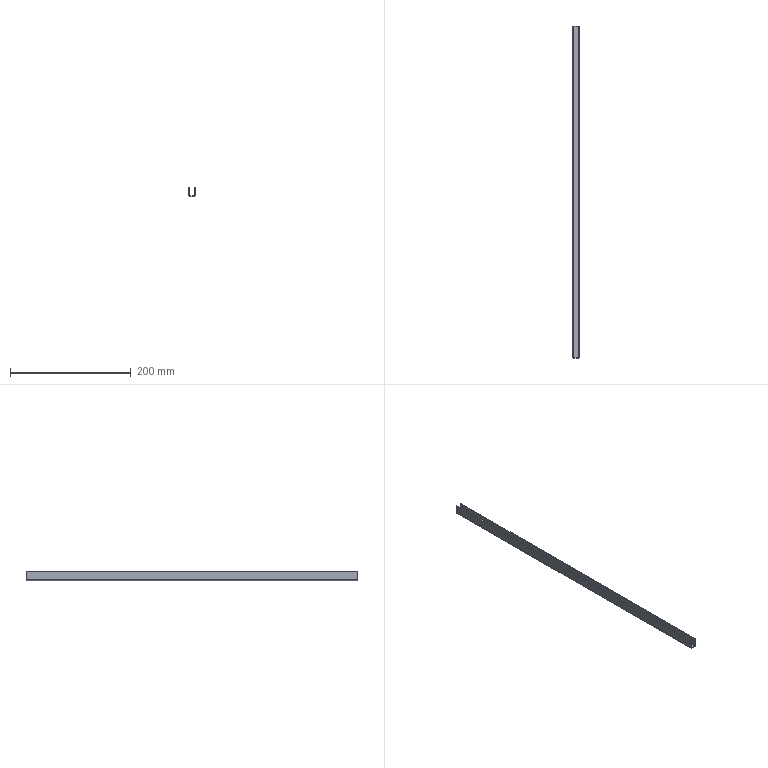Part | SolidWorks | features EdgeFlange 1, FlatPattern 1, SMBaseFlange 1, SheetMetal 1 | 1 solid | 22 faces | box 10.4 x 550 x 15 mm | volume 24485 mm3 | plane 18 | cylinder 4 | commonest cylinder face diameters 0.9 x2 3.3 x2
STEP:
#1=CARTESIAN_POINT('',(-11.654,-507.682,1.2));
#2=VERTEX_POINT('',#1);
#3=CARTESIAN_POINT('',(-11.654,-507.682,0.));
#4=VERTEX_POINT('',#3);
#5=CARTESIAN_POINT('',(-11.654,-507.682,1.2));
#6=DIRECTION('',(0.,0.,-1.));
#7=VECTOR('',#6,1000.);
#8=LINE('',#5,#7);
#9=EDGE_CURVE('',#2,#4,#8,.T.);
#10=ORIENTED_EDGE('',*,*,#9,.T.);
#11=CARTESIAN_POINT('',(-4.554,-507.682,0.));
#12=VERTEX_POINT('',#11);
#13=CARTESIAN_POINT('',(-13.304,-507.682,0.));
#14=DIRECTION('',(1.,0.,0.));
#15=VECTOR('',#14,1000.);
#16=LINE('',#13,#15);
#17=EDGE_CURVE('',#4,#12,#16,.T.);
#18=ORIENTED_EDGE('',*,*,#17,.T.);
#19=CARTESIAN_POINT('',(-4.554,-507.682,1.2));
#20=VERTEX_POINT('',#19);
#21=CARTESIAN_POINT('',(-4.554,-507.682,1.2));
#22=DIRECTION('',(0.,0.,-1.));
#23=VECTOR('',#22,1000.);
#24=LINE('',#21,#23);
#25=EDGE_CURVE('',#20,#12,#24,.T.);
#26=ORIENTED_EDGE('',*,*,#25,.F.);
#27=CARTESIAN_POINT('',(-13.304,-507.682,1.2));
#28=DIRECTION('',(1.,0.,0.));
#29=VECTOR('',#28,1000.);
#30=LINE('',#27,#29);
#31=EDGE_CURVE('',#2,#20,#30,.T.);
#32=ORIENTED_EDGE('',*,*,#31,.F.);
#33=EDGE_LOOP('',(#10,#18,#26,#32));
#34=FACE_OUTER_BOUND('',#33,.T.);
#35=CARTESIAN_POINT('',(-13.304,-507.682,1.2));
#36=DIRECTION('',(0.,1.,0.));
#37=DIRECTION('',(0.,0.,1.));
#38=AXIS2_PLACEMENT_3D('',#35,#36,#37);
#39=PLANE('',#38);
#40=ADVANCED_FACE('',(#34),#39,.F.);
#41=CARTESIAN_POINT('',(-11.654,42.318,1.2));
#42=VERTEX_POINT('',#41);
#43=CARTESIAN_POINT('',(-11.654,42.318,0.));
#44=VERTEX_POINT('',#43);
#45=CARTESIAN_POINT('',(-11.654,42.318,1.2));
#46=DIRECTION('',(0.,0.,-1.));
#47=VECTOR('',#46,1000.);
#48=LINE('',#45,#47);
#49=EDGE_CURVE('',#42,#44,#48,.T.);
#50=ORIENTED_EDGE('',*,*,#49,.F.);
#51=CARTESIAN_POINT('',(-4.554,42.318,1.2));
#52=VERTEX_POINT('',#51);
#53=CARTESIAN_POINT('',(-13.304,42.318,1.2));
#54=DIRECTION('',(-1.,0.,0.));
#55=VECTOR('',#54,1000.);
#56=LINE('',#53,#55);
#57=EDGE_CURVE('',#52,#42,#56,.T.);
#58=ORIENTED_EDGE('',*,*,#57,.F.);
#59=CARTESIAN_POINT('',(-4.554,42.318,0.));
#60=VERTEX_POINT('',#59);
#61=CARTESIAN_POINT('',(-4.554,42.318,1.2));
#62=DIRECTION('',(0.,0.,-1.));
#63=VECTOR('',#62,1000.);
#64=LINE('',#61,#63);
#65=EDGE_CURVE('',#52,#60,#64,.T.);
#66=ORIENTED_EDGE('',*,*,#65,.T.);
#67=CARTESIAN_POINT('',(-13.304,42.318,0.));
#68=DIRECTION('',(-1.,0.,0.));
#69=VECTOR('',#68,1000.);
#70=LINE('',#67,#69);
#71=EDGE_CURVE('',#60,#44,#70,.T.);
#72=ORIENTED_EDGE('',*,*,#71,.T.);
#73=EDGE_LOOP('',(#50,#58,#66,#72));
#74=FACE_OUTER_BOUND('',#73,.T.);
#75=CARTESIAN_POINT('',(-13.304,42.318,1.2));
#76=DIRECTION('',(0.,-1.,0.));
#77=DIRECTION('',(0.,0.,-1.));
#78=AXIS2_PLACEMENT_3D('',#75,#76,#77);
#79=PLANE('',#78);
#80=ADVANCED_FACE('',(#74),#79,.F.);
#81=ORIENTED_EDGE('',*,*,#57,.T.);
#82=CARTESIAN_POINT('',(-11.654,-507.682,1.2));
#83=DIRECTION('',(0.,1.,0.));
#84=VECTOR('',#83,1000.);
#85=LINE('',#82,#84);
#86=EDGE_CURVE('',#2,#42,#85,.T.);
#87=ORIENTED_EDGE('',*,*,#86,.F.);
#88=ORIENTED_EDGE('',*,*,#31,.T.);
#89=CARTESIAN_POINT('',(-4.554,42.318,1.2));
#90=DIRECTION('',(0.,-1.,0.));
#91=VECTOR('',#90,1000.);
#92=LINE('',#89,#91);
#93=EDGE_CURVE('',#52,#20,#92,.T.);
#94=ORIENTED_EDGE('',*,*,#93,.F.);
#95=EDGE_LOOP('',(#81,#87,#88,#94));
#96=FACE_OUTER_BOUND('',#95,.T.);
#97=CARTESIAN_POINT('',(-13.304,-507.682,1.2));
#98=DIRECTION('',(0.,0.,1.));
#99=DIRECTION('',(1.,0.,0.));
#100=AXIS2_PLACEMENT_3D('',#97,#98,#99);
#101=PLANE('',#100);
#102=ADVANCED_FACE('',(#96),#101,.T.);
#103=CARTESIAN_POINT('',(-11.654,-507.682,0.));
#104=DIRECTION('',(0.,1.,0.));
#105=VECTOR('',#104,1000.);
#106=LINE('',#103,#105);
#107=EDGE_CURVE('',#4,#44,#106,.T.);
#108=ORIENTED_EDGE('',*,*,#107,.T.);
#109=ORIENTED_EDGE('',*,*,#71,.F.);
#110=CARTESIAN_POINT('',(-4.554,42.318,0.));
#111=DIRECTION('',(0.,-1.,0.));
#112=VECTOR('',#111,1000.);
#113=LINE('',#110,#112);
#114=EDGE_CURVE('',#60,#12,#113,.T.);
#115=ORIENTED_EDGE('',*,*,#114,.T.);
#116=ORIENTED_EDGE('',*,*,#17,.F.);
#117=EDGE_LOOP('',(#108,#109,#115,#116));
#118=FACE_OUTER_BOUND('',#117,.T.);
#119=CARTESIAN_POINT('',(-13.304,-507.682,0.));
#120=DIRECTION('',(0.,0.,1.));
#121=DIRECTION('',(1.,0.,0.));
#122=AXIS2_PLACEMENT_3D('',#119,#120,#121);
#123=PLANE('',#122);
#124=ADVANCED_FACE('',(#118),#123,.F.);
#125=CARTESIAN_POINT('',(-4.104,-507.682,1.65));
#126=VERTEX_POINT('',#125);
#127=CARTESIAN_POINT('',(-2.904,-507.682,1.65));
#128=VERTEX_POINT('',#127);
#129=CARTESIAN_POINT('',(-2.904,-507.682,1.65));
#130=DIRECTION('',(1.,0.,0.));
#131=VECTOR('',#130,1000.);
#132=LINE('',#129,#131);
#133=EDGE_CURVE('',#126,#128,#132,.T.);
#134=ORIENTED_EDGE('',*,*,#133,.F.);
#135=CARTESIAN_POINT('',(-4.554,-507.682,1.65));
#136=DIRECTION('',(0.,-1.,0.));
#137=DIRECTION('',(0.,0.,1.));
#138=AXIS2_PLACEMENT_3D('',#135,#136,#137);
#139=CIRCLE('',#138,0.45);
#140=EDGE_CURVE('',#20,#126,#139,.T.);
#141=ORIENTED_EDGE('',*,*,#140,.F.);
#142=ORIENTED_EDGE('',*,*,#25,.T.);
#143=CARTESIAN_POINT('',(-4.554,-507.682,1.65));
#144=DIRECTION('',(0.,-1.,0.));
#145=DIRECTION('',(0.,0.,1.));
#146=AXIS2_PLACEMENT_3D('',#143,#144,#145);
#147=CIRCLE('',#146,1.65);
#148=EDGE_CURVE('',#12,#128,#147,.T.);
#149=ORIENTED_EDGE('',*,*,#148,.T.);
#150=EDGE_LOOP('',(#134,#141,#142,#149));
#151=FACE_OUTER_BOUND('',#150,.T.);
#152=CARTESIAN_POINT('',(-4.554,-507.682,1.65));
#153=DIRECTION('',(0.,-1.,0.));
#154=DIRECTION('',(0.,0.,-1.));
#155=AXIS2_PLACEMENT_3D('',#152,#153,#154);
#156=PLANE('',#155);
#157=ADVANCED_FACE('',(#151),#156,.T.);
#158=ORIENTED_EDGE('',*,*,#114,.F.);
#159=CARTESIAN_POINT('',(-2.904,42.318,1.65));
#160=VERTEX_POINT('',#159);
#161=CARTESIAN_POINT('',(-4.554,42.318,1.65));
#162=DIRECTION('',(0.,1.,0.));
#163=DIRECTION('',(0.,0.,1.));
#164=AXIS2_PLACEMENT_3D('',#161,#162,#163);
#165=CIRCLE('',#164,1.65);
#166=EDGE_CURVE('',#160,#60,#165,.T.);
#167=ORIENTED_EDGE('',*,*,#166,.F.);
#168=CARTESIAN_POINT('',(-2.904,-507.682,1.65));
#169=DIRECTION('',(0.,-1.,0.));
#170=VECTOR('',#169,1000.);
#171=LINE('',#168,#170);
#172=EDGE_CURVE('',#160,#128,#171,.T.);
#173=ORIENTED_EDGE('',*,*,#172,.T.);
#174=ORIENTED_EDGE('',*,*,#148,.F.);
#175=EDGE_LOOP('',(#158,#167,#173,#174));
#176=FACE_OUTER_BOUND('',#175,.T.);
#177=CARTESIAN_POINT('',(-4.554,42.318,1.65));
#178=DIRECTION('',(0.,1.,0.));
#179=DIRECTION('',(1.,0.,0.));
#180=AXIS2_PLACEMENT_3D('',#177,#178,#179);
#181=CYLINDRICAL_SURFACE('',#180,1.65);
#182=ADVANCED_FACE('',(#176),#181,.T.);
#183=CARTESIAN_POINT('',(-4.104,42.318,1.65));
#184=VERTEX_POINT('',#183);
#185=CARTESIAN_POINT('',(-4.554,42.318,1.65));
#186=DIRECTION('',(0.,1.,0.));
#187=DIRECTION('',(0.,0.,1.));
#188=AXIS2_PLACEMENT_3D('',#185,#186,#187);
#189=CIRCLE('',#188,0.45);
#190=EDGE_CURVE('',#184,#52,#189,.T.);
#191=ORIENTED_EDGE('',*,*,#190,.F.);
#192=CARTESIAN_POINT('',(-4.104,42.318,1.65));
#193=DIRECTION('',(1.,0.,0.));
#194=VECTOR('',#193,1000.);
#195=LINE('',#192,#194);
#196=EDGE_CURVE('',#184,#160,#195,.T.);
#197=ORIENTED_EDGE('',*,*,#196,.T.);
#198=ORIENTED_EDGE('',*,*,#166,.T.);
#199=ORIENTED_EDGE('',*,*,#65,.F.);
#200=EDGE_LOOP('',(#191,#197,#198,#199));
#201=FACE_OUTER_BOUND('',#200,.T.);
#202=CARTESIAN_POINT('',(-4.554,42.318,1.65));
#203=DIRECTION('',(0.,-1.,0.));
#204=DIRECTION('',(0.,0.,-1.));
#205=AXIS2_PLACEMENT_3D('',#202,#203,#204);
#206=PLANE('',#205);
#207=ADVANCED_FACE('',(#201),#206,.F.);
#208=ORIENTED_EDGE('',*,*,#93,.T.);
#209=ORIENTED_EDGE('',*,*,#140,.T.);
#210=CARTESIAN_POINT('',(-4.104,-507.682,1.65));
#211=DIRECTION('',(0.,1.,0.));
#212=VECTOR('',#211,1000.);
#213=LINE('',#210,#212);
#214=EDGE_CURVE('',#126,#184,#213,.T.);
#215=ORIENTED_EDGE('',*,*,#214,.T.);
#216=ORIENTED_EDGE('',*,*,#190,.T.);
#217=EDGE_LOOP('',(#208,#209,#215,#216));
#218=FACE_OUTER_BOUND('',#217,.T.);
#219=CARTESIAN_POINT('',(-4.554,42.318,1.65));
#220=DIRECTION('',(0.,1.,0.));
#221=DIRECTION('',(1.,0.,0.));
#222=AXIS2_PLACEMENT_3D('',#219,#220,#221);
#223=CYLINDRICAL_SURFACE('',#222,0.45);
#224=ADVANCED_FACE('',(#218),#223,.F.);
#225=ORIENTED_EDGE('',*,*,#196,.F.);
#226=CARTESIAN_POINT('',(-4.104,42.318,15.));
#227=VERTEX_POINT('',#226);
#228=CARTESIAN_POINT('',(-4.104,42.318,15.));
#229=DIRECTION('',(0.,0.,1.));
#230=VECTOR('',#229,1000.);
#231=LINE('',#228,#230);
#232=EDGE_CURVE('',#184,#227,#231,.T.);
#233=ORIENTED_EDGE('',*,*,#232,.T.);
#234=CARTESIAN_POINT('',(-2.904,42.318,15.));
#235=VERTEX_POINT('',#234);
#236=CARTESIAN_POINT('',(-2.904,42.318,15.));
#237=DIRECTION('',(-1.,0.,0.));
#238=VECTOR('',#237,1000.);
#239=LINE('',#236,#238);
#240=EDGE_CURVE('',#235,#227,#239,.T.);
#241=ORIENTED_EDGE('',*,*,#240,.F.);
#242=CARTESIAN_POINT('',(-2.904,42.318,1.2));
#243=DIRECTION('',(0.,0.,1.));
#244=VECTOR('',#243,1000.);
#245=LINE('',#242,#244);
#246=EDGE_CURVE('',#160,#235,#245,.T.);
#247=ORIENTED_EDGE('',*,*,#246,.F.);
#248=EDGE_LOOP('',(#225,#233,#241,#247));
#249=FACE_OUTER_BOUND('',#248,.T.);
#250=CARTESIAN_POINT('',(-2.904,42.318,15.));
#251=DIRECTION('',(0.,-1.,0.));
#252=DIRECTION('',(1.,0.,0.));
#253=AXIS2_PLACEMENT_3D('',#250,#251,#252);
#254=PLANE('',#253);
#255=ADVANCED_FACE('',(#249),#254,.F.);
#256=ORIENTED_EDGE('',*,*,#133,.T.);
#257=CARTESIAN_POINT('',(-2.904,-507.682,15.));
#258=VERTEX_POINT('',#257);
#259=CARTESIAN_POINT('',(-2.904,-507.682,1.2));
#260=DIRECTION('',(0.,0.,-1.));
#261=VECTOR('',#260,1000.);
#262=LINE('',#259,#261);
#263=EDGE_CURVE('',#258,#128,#262,.T.);
#264=ORIENTED_EDGE('',*,*,#263,.F.);
#265=CARTESIAN_POINT('',(-4.104,-507.682,15.));
#266=VERTEX_POINT('',#265);
#267=CARTESIAN_POINT('',(-2.904,-507.682,15.));
#268=DIRECTION('',(-1.,0.,0.));
#269=VECTOR('',#268,1000.);
#270=LINE('',#267,#269);
#271=EDGE_CURVE('',#258,#266,#270,.T.);
#272=ORIENTED_EDGE('',*,*,#271,.T.);
#273=CARTESIAN_POINT('',(-4.104,-507.682,1.2));
#274=DIRECTION('',(0.,0.,-1.));
#275=VECTOR('',#274,1000.);
#276=LINE('',#273,#275);
#277=EDGE_CURVE('',#266,#126,#276,.T.);
#278=ORIENTED_EDGE('',*,*,#277,.T.);
#279=EDGE_LOOP('',(#256,#264,#272,#278));
#280=FACE_OUTER_BOUND('',#279,.T.);
#281=CARTESIAN_POINT('',(-2.904,-507.682,1.2));
#282=DIRECTION('',(0.,1.,0.));
#283=DIRECTION('',(-1.,0.,0.));
#284=AXIS2_PLACEMENT_3D('',#281,#282,#283);
#285=PLANE('',#284);
#286=ADVANCED_FACE('',(#280),#285,.F.);
#287=ORIENTED_EDGE('',*,*,#172,.F.);
#288=ORIENTED_EDGE('',*,*,#246,.T.);
#289=CARTESIAN_POINT('',(-2.904,42.318,15.));
#290=DIRECTION('',(0.,-1.,0.));
#291=VECTOR('',#290,1000.);
#292=LINE('',#289,#291);
#293=EDGE_CURVE('',#235,#258,#292,.T.);
#294=ORIENTED_EDGE('',*,*,#293,.T.);
#295=ORIENTED_EDGE('',*,*,#263,.T.);
#296=EDGE_LOOP('',(#287,#288,#294,#295));
#297=FACE_OUTER_BOUND('',#296,.T.);
#298=CARTESIAN_POINT('',(-2.904,42.318,1.2));
#299=DIRECTION('',(-1.,0.,0.));
#300=DIRECTION('',(0.,0.,1.));
#301=AXIS2_PLACEMENT_3D('',#298,#299,#300);
#302=PLANE('',#301);
#303=ADVANCED_FACE('',(#297),#302,.F.);
#304=ORIENTED_EDGE('',*,*,#232,.F.);
#305=ORIENTED_EDGE('',*,*,#214,.F.);
#306=ORIENTED_EDGE('',*,*,#277,.F.);
#307=CARTESIAN_POINT('',(-4.104,-507.682,15.));
#308=DIRECTION('',(0.,-1.,0.));
#309=VECTOR('',#308,1000.);
#310=LINE('',#307,#309);
#311=EDGE_CURVE('',#227,#266,#310,.T.);
#312=ORIENTED_EDGE('',*,*,#311,.F.);
#313=EDGE_LOOP('',(#304,#305,#306,#312));
#314=FACE_OUTER_BOUND('',#313,.T.);
#315=CARTESIAN_POINT('',(-4.104,42.318,1.2));
#316=DIRECTION('',(-1.,0.,0.));
#317=DIRECTION('',(0.,0.,1.));
#318=AXIS2_PLACEMENT_3D('',#315,#316,#317);
#319=PLANE('',#318);
#320=ADVANCED_FACE('',(#314),#319,.T.);
#321=ORIENTED_EDGE('',*,*,#311,.T.);
#322=ORIENTED_EDGE('',*,*,#271,.F.);
#323=ORIENTED_EDGE('',*,*,#293,.F.);
#324=ORIENTED_EDGE('',*,*,#240,.T.);
#325=EDGE_LOOP('',(#321,#322,#323,#324));
#326=FACE_OUTER_BOUND('',#325,.T.);
#327=CARTESIAN_POINT('',(-2.904,-507.682,15.));
#328=DIRECTION('',(0.,0.,-1.));
#329=DIRECTION('',(-1.,0.,0.));
#330=AXIS2_PLACEMENT_3D('',#327,#328,#329);
#331=PLANE('',#330);
#332=ADVANCED_FACE('',(#326),#331,.F.);
#333=CARTESIAN_POINT('',(-12.104,42.318,1.65));
#334=VERTEX_POINT('',#333);
#335=CARTESIAN_POINT('',(-13.304,42.318,1.65));
#336=VERTEX_POINT('',#335);
#337=CARTESIAN_POINT('',(-13.304,42.318,1.65));
#338=DIRECTION('',(-1.,0.,0.));
#339=VECTOR('',#338,1000.);
#340=LINE('',#337,#339);
#341=EDGE_CURVE('',#334,#336,#340,.T.);
#342=ORIENTED_EDGE('',*,*,#341,.F.);
#343=CARTESIAN_POINT('',(-11.654,42.318,1.65));
#344=DIRECTION('',(0.,1.,0.));
#345=DIRECTION('',(0.,0.,-1.));
#346=AXIS2_PLACEMENT_3D('',#343,#344,#345);
#347=CIRCLE('',#346,0.45);
#348=EDGE_CURVE('',#42,#334,#347,.T.);
#349=ORIENTED_EDGE('',*,*,#348,.F.);
#350=ORIENTED_EDGE('',*,*,#49,.T.);
#351=CARTESIAN_POINT('',(-11.654,42.318,1.65));
#352=DIRECTION('',(0.,1.,0.));
#353=DIRECTION('',(0.,0.,-1.));
#354=AXIS2_PLACEMENT_3D('',#351,#352,#353);
#355=CIRCLE('',#354,1.65);
#356=EDGE_CURVE('',#44,#336,#355,.T.);
#357=ORIENTED_EDGE('',*,*,#356,.T.);
#358=EDGE_LOOP('',(#342,#349,#350,#357));
#359=FACE_OUTER_BOUND('',#358,.T.);
#360=CARTESIAN_POINT('',(-11.654,42.318,1.65));
#361=DIRECTION('',(0.,1.,0.));
#362=DIRECTION('',(0.,0.,1.));
#363=AXIS2_PLACEMENT_3D('',#360,#361,#362);
#364=PLANE('',#363);
#365=ADVANCED_FACE('',(#359),#364,.T.);
#366=ORIENTED_EDGE('',*,*,#107,.F.);
#367=CARTESIAN_POINT('',(-13.304,-507.682,1.65));
#368=VERTEX_POINT('',#367);
#369=CARTESIAN_POINT('',(-11.654,-507.682,1.65));
#370=DIRECTION('',(0.,-1.,0.));
#371=DIRECTION('',(0.,0.,-1.));
#372=AXIS2_PLACEMENT_3D('',#369,#370,#371);
#373=CIRCLE('',#372,1.65);
#374=EDGE_CURVE('',#368,#4,#373,.T.);
#375=ORIENTED_EDGE('',*,*,#374,.F.);
#376=CARTESIAN_POINT('',(-13.304,42.318,1.65));
#377=DIRECTION('',(0.,1.,0.));
#378=VECTOR('',#377,1000.);
#379=LINE('',#376,#378);
#380=EDGE_CURVE('',#368,#336,#379,.T.);
#381=ORIENTED_EDGE('',*,*,#380,.T.);
#382=ORIENTED_EDGE('',*,*,#356,.F.);
#383=EDGE_LOOP('',(#366,#375,#381,#382));
#384=FACE_OUTER_BOUND('',#383,.T.);
#385=CARTESIAN_POINT('',(-11.654,-507.682,1.65));
#386=DIRECTION('',(0.,-1.,0.));
#387=DIRECTION('',(-1.,0.,0.));
#388=AXIS2_PLACEMENT_3D('',#385,#386,#387);
#389=CYLINDRICAL_SURFACE('',#388,1.65);
#390=ADVANCED_FACE('',(#384),#389,.T.);
#391=CARTESIAN_POINT('',(-12.104,-507.682,1.65));
#392=VERTEX_POINT('',#391);
#393=CARTESIAN_POINT('',(-11.654,-507.682,1.65));
#394=DIRECTION('',(0.,-1.,0.));
#395=DIRECTION('',(0.,0.,-1.));
#396=AXIS2_PLACEMENT_3D('',#393,#394,#395);
#397=CIRCLE('',#396,0.45);
#398=EDGE_CURVE('',#392,#2,#397,.T.);
#399=ORIENTED_EDGE('',*,*,#398,.F.);
#400=CARTESIAN_POINT('',(-12.104,-507.682,1.65));
#401=DIRECTION('',(-1.,0.,0.));
#402=VECTOR('',#401,1000.);
#403=LINE('',#400,#402);
#404=EDGE_CURVE('',#392,#368,#403,.T.);
#405=ORIENTED_EDGE('',*,*,#404,.T.);
#406=ORIENTED_EDGE('',*,*,#374,.T.);
#407=ORIENTED_EDGE('',*,*,#9,.F.);
#408=EDGE_LOOP('',(#399,#405,#406,#407));
#409=FACE_OUTER_BOUND('',#408,.T.);
#410=CARTESIAN_POINT('',(-11.654,-507.682,1.65));
#411=DIRECTION('',(0.,1.,0.));
#412=DIRECTION('',(0.,0.,1.));
#413=AXIS2_PLACEMENT_3D('',#410,#411,#412);
#414=PLANE('',#413);
#415=ADVANCED_FACE('',(#409),#414,.F.);
#416=ORIENTED_EDGE('',*,*,#86,.T.);
#417=ORIENTED_EDGE('',*,*,#348,.T.);
#418=CARTESIAN_POINT('',(-12.104,42.318,1.65));
#419=DIRECTION('',(0.,-1.,0.));
#420=VECTOR('',#419,1000.);
#421=LINE('',#418,#420);
#422=EDGE_CURVE('',#334,#392,#421,.T.);
#423=ORIENTED_EDGE('',*,*,#422,.T.);
#424=ORIENTED_EDGE('',*,*,#398,.T.);
#425=EDGE_LOOP('',(#416,#417,#423,#424));
#426=FACE_OUTER_BOUND('',#425,.T.);
#427=CARTESIAN_POINT('',(-11.654,-507.682,1.65));
#428=DIRECTION('',(0.,-1.,0.));
#429=DIRECTION('',(-1.,0.,0.));
#430=AXIS2_PLACEMENT_3D('',#427,#428,#429);
#431=CYLINDRICAL_SURFACE('',#430,0.45);
#432=ADVANCED_FACE('',(#426),#431,.F.);
#433=ORIENTED_EDGE('',*,*,#341,.T.);
#434=CARTESIAN_POINT('',(-13.304,42.318,15.));
#435=VERTEX_POINT('',#434);
#436=CARTESIAN_POINT('',(-13.304,42.318,15.));
#437=DIRECTION('',(0.,0.,-1.));
#438=VECTOR('',#437,1000.);
#439=LINE('',#436,#438);
#440=EDGE_CURVE('',#435,#336,#439,.T.);
#441=ORIENTED_EDGE('',*,*,#440,.F.);
#442=CARTESIAN_POINT('',(-12.104,42.318,15.));
#443=VERTEX_POINT('',#442);
#444=CARTESIAN_POINT('',(-13.304,42.318,15.));
#445=DIRECTION('',(1.,0.,0.));
#446=VECTOR('',#445,1000.);
#447=LINE('',#444,#446);
#448=EDGE_CURVE('',#435,#443,#447,.T.);
#449=ORIENTED_EDGE('',*,*,#448,.T.);
#450=CARTESIAN_POINT('',(-12.104,42.318,1.2));
#451=DIRECTION('',(0.,0.,-1.));
#452=VECTOR('',#451,1000.);
#453=LINE('',#450,#452);
#454=EDGE_CURVE('',#443,#334,#453,.T.);
#455=ORIENTED_EDGE('',*,*,#454,.T.);
#456=EDGE_LOOP('',(#433,#441,#449,#455));
#457=FACE_OUTER_BOUND('',#456,.T.);
#458=CARTESIAN_POINT('',(-13.304,42.318,1.2));
#459=DIRECTION('',(0.,-1.,0.));
#460=DIRECTION('',(1.,0.,0.));
#461=AXIS2_PLACEMENT_3D('',#458,#459,#460);
#462=PLANE('',#461);
#463=ADVANCED_FACE('',(#457),#462,.F.);
#464=ORIENTED_EDGE('',*,*,#404,.F.);
#465=CARTESIAN_POINT('',(-12.104,-507.682,15.));
#466=VERTEX_POINT('',#465);
#467=CARTESIAN_POINT('',(-12.104,-507.682,15.));
#468=DIRECTION('',(0.,0.,1.));
#469=VECTOR('',#468,1000.);
#470=LINE('',#467,#469);
#471=EDGE_CURVE('',#392,#466,#470,.T.);
#472=ORIENTED_EDGE('',*,*,#471,.T.);
#473=CARTESIAN_POINT('',(-13.304,-507.682,15.));
#474=VERTEX_POINT('',#473);
#475=CARTESIAN_POINT('',(-13.304,-507.682,15.));
#476=DIRECTION('',(1.,0.,0.));
#477=VECTOR('',#476,1000.);
#478=LINE('',#475,#477);
#479=EDGE_CURVE('',#474,#466,#478,.T.);
#480=ORIENTED_EDGE('',*,*,#479,.F.);
#481=CARTESIAN_POINT('',(-13.304,-507.682,15.));
#482=DIRECTION('',(0.,0.,1.));
#483=VECTOR('',#482,1000.);
#484=LINE('',#481,#483);
#485=EDGE_CURVE('',#368,#474,#484,.T.);
#486=ORIENTED_EDGE('',*,*,#485,.F.);
#487=EDGE_LOOP('',(#464,#472,#480,#486));
#488=FACE_OUTER_BOUND('',#487,.T.);
#489=CARTESIAN_POINT('',(-13.304,-507.682,15.));
#490=DIRECTION('',(0.,1.,0.));
#491=DIRECTION('',(-1.,0.,0.));
#492=AXIS2_PLACEMENT_3D('',#489,#490,#491);
#493=PLANE('',#492);
#494=ADVANCED_FACE('',(#488),#493,.F.);
#495=ORIENTED_EDGE('',*,*,#380,.F.);
#496=ORIENTED_EDGE('',*,*,#485,.T.);
#497=CARTESIAN_POINT('',(-13.304,42.318,15.));
#498=DIRECTION('',(0.,1.,0.));
#499=VECTOR('',#498,1000.);
#500=LINE('',#497,#499);
#501=EDGE_CURVE('',#474,#435,#500,.T.);
#502=ORIENTED_EDGE('',*,*,#501,.T.);
#503=ORIENTED_EDGE('',*,*,#440,.T.);
#504=EDGE_LOOP('',(#495,#496,#502,#503));
#505=FACE_OUTER_BOUND('',#504,.T.);
#506=CARTESIAN_POINT('',(-13.304,42.318,15.));
#507=DIRECTION('',(1.,0.,0.));
#508=DIRECTION('',(0.,0.,-1.));
#509=AXIS2_PLACEMENT_3D('',#506,#507,#508);
#510=PLANE('',#509);
#511=ADVANCED_FACE('',(#505),#510,.F.);
#512=ORIENTED_EDGE('',*,*,#471,.F.);
#513=ORIENTED_EDGE('',*,*,#422,.F.);
#514=ORIENTED_EDGE('',*,*,#454,.F.);
#515=CARTESIAN_POINT('',(-12.104,42.318,15.));
#516=DIRECTION('',(0.,1.,0.));
#517=VECTOR('',#516,1000.);
#518=LINE('',#515,#517);
#519=EDGE_CURVE('',#466,#443,#518,.T.);
#520=ORIENTED_EDGE('',*,*,#519,.F.);
#521=EDGE_LOOP('',(#512,#513,#514,#520));
#522=FACE_OUTER_BOUND('',#521,.T.);
#523=CARTESIAN_POINT('',(-12.104,42.318,15.));
#524=DIRECTION('',(1.,0.,0.));
#525=DIRECTION('',(0.,0.,-1.));
#526=AXIS2_PLACEMENT_3D('',#523,#524,#525);
#527=PLANE('',#526);
#528=ADVANCED_FACE('',(#522),#527,.T.);
#529=ORIENTED_EDGE('',*,*,#519,.T.);
#530=ORIENTED_EDGE('',*,*,#448,.F.);
#531=ORIENTED_EDGE('',*,*,#501,.F.);
#532=ORIENTED_EDGE('',*,*,#479,.T.);
#533=EDGE_LOOP('',(#529,#530,#531,#532));
#534=FACE_OUTER_BOUND('',#533,.T.);
#535=CARTESIAN_POINT('',(-13.304,42.318,15.));
#536=DIRECTION('',(0.,0.,-1.));
#537=DIRECTION('',(-1.,0.,0.));
#538=AXIS2_PLACEMENT_3D('',#535,#536,#537);
#539=PLANE('',#538);
#540=ADVANCED_FACE('',(#534),#539,.F.);
#541=CLOSED_SHELL('',(#40,#80,#102,#124,#157,#182,#207,#224,#255,#286,#303,#320,#332,#365,#390,#415,#432,#463,#494,#511,#528,#540));
#542=MANIFOLD_SOLID_BREP('',#541);
#543=CARTESIAN_POINT('',(0.,0.,0.));
#544=DIRECTION('',(0.,0.,1.));
#545=DIRECTION('',(1.,0.,0.));
#546=AXIS2_PLACEMENT_3D('',#543,#544,#545);
#547=(LENGTH_UNIT()NAMED_UNIT(*)SI_UNIT(.MILLI.,.METRE.));
#548=UNCERTAINTY_MEASURE_WITH_UNIT(LENGTH_MEASURE(0.00001),#547,'','');
#549=(NAMED_UNIT(*)PLANE_ANGLE_UNIT()SI_UNIT($,.RADIAN.));
#550=(NAMED_UNIT(*)SI_UNIT($,.STERADIAN.)SOLID_ANGLE_UNIT());
#551=(GEOMETRIC_REPRESENTATION_CONTEXT(3)GLOBAL_UNCERTAINTY_ASSIGNED_CONTEXT((#548))GLOBAL_UNIT_ASSIGNED_CONTEXT((#547,#549,#550))REPRESENTATION_CONTEXT('',''));
#552=ADVANCED_BREP_SHAPE_REPRESENTATION('',(#542,#546),#551);